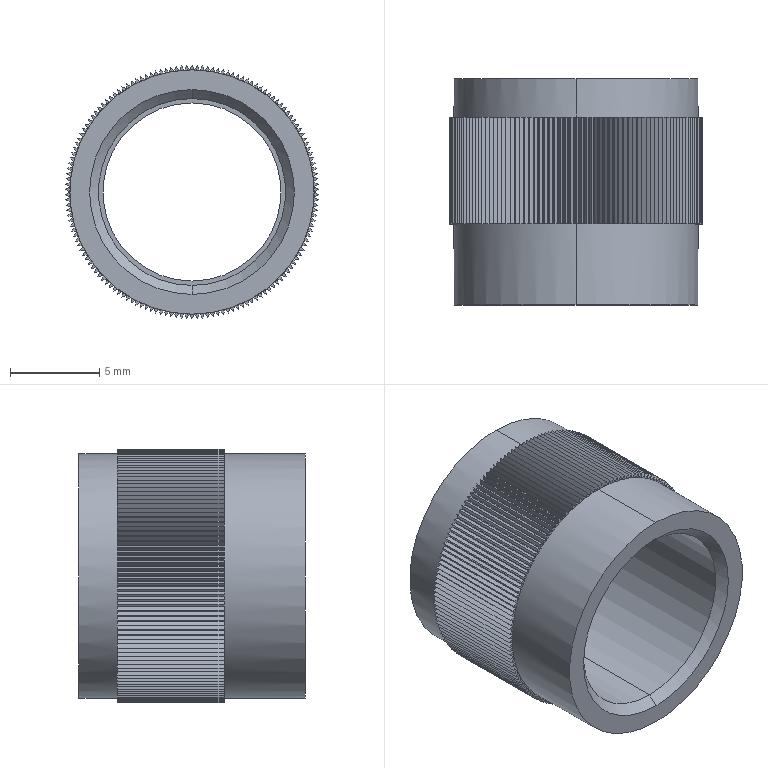Part | SolidWorks | features Chamfer 1, ICE 1, Revolution 1 | 1 solid | 611 faces | box 14.217 x 12.7 x 14.22 mm | volume 809.778 mm3 | plane 603 | cylinder 6 | cone 2 | commonest cylinder face diameters 10 x2 10.5 x2 13.72 x2